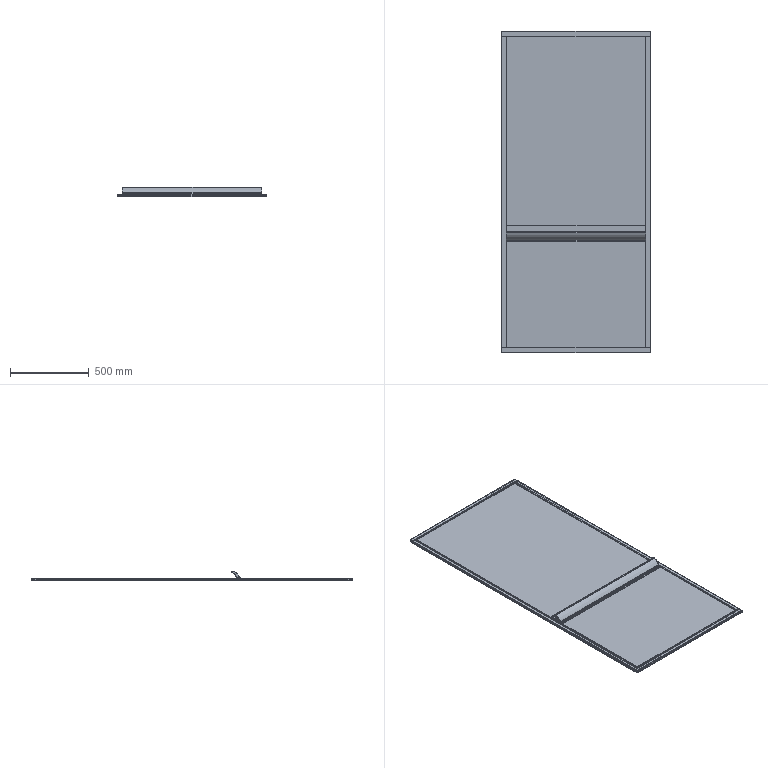Part | 13 solids | 408 faces | box 940 x 2036 x 62.186 mm | volume 19081318 mm3 | plane 252 | cylinder 156 | commonest cylinder face diameters 1.1 x36 3.6 x32 5.8 x29 4 x24 1 x10 0.4 x8